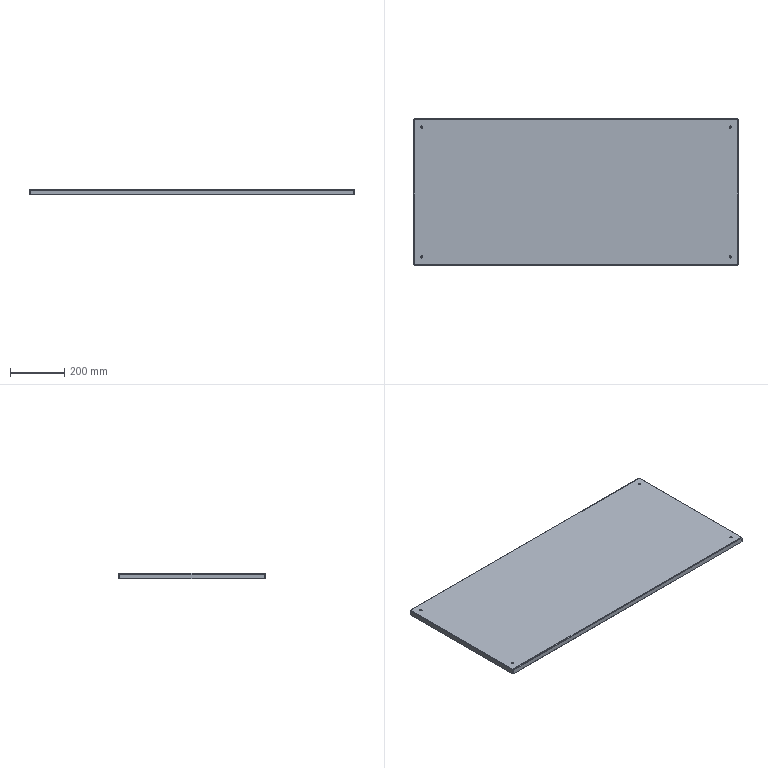Part | STEP file | 09-22 electrical control board | 1 solid | 46 faces | box 1200 x 540 x 20 mm | volume 1414884 mm3 | plane 22 | cylinder 16 | spline 8 | commonest cylinder face diameters 8 x8 1.473 x4 5.473 x4